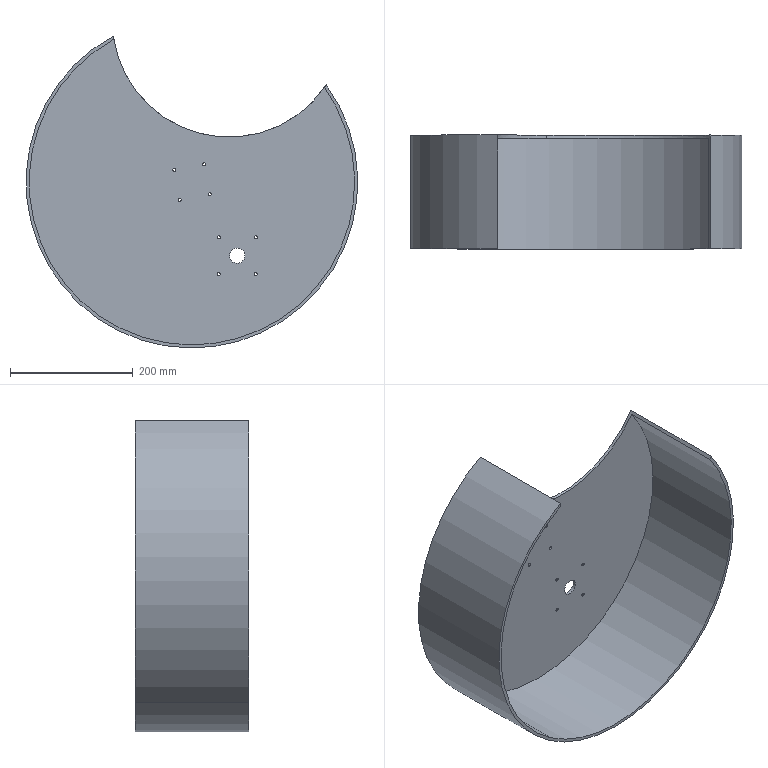Part | STEP file | Cut-Extrude 6-1 | 1 solid | 27 faces | box 540 x 185 x 507.759 mm | volume 2066014 mm3 | cylinder 24 | plane 3 | commonest cylinder face diameters 5 x16 25 x2 380 x2 530 x2 540 x2
STEP:
#1=CARTESIAN_POINT('',(-1346.779,1658.264,3090.615));
#2=VERTEX_POINT('',#1);
#3=CARTESIAN_POINT('',(-1713.217,1658.264,2718.76));
#4=VERTEX_POINT('',#3);
#5=CARTESIAN_POINT('',(-1562.535,1658.264,2936.751));
#6=DIRECTION('',(0.,1.,0.));
#7=DIRECTION('',(-0.5686,0.,-0.8226));
#8=AXIS2_PLACEMENT_3D('',#5,#6,#7);
#9=CIRCLE('',#8,265.);
#10=EDGE_CURVE('',#2,#4,#9,.T.);
#11=ORIENTED_EDGE('',*,*,#10,.T.);
#12=CARTESIAN_POINT('',(-1713.217,1478.264,2718.76));
#13=VERTEX_POINT('',#12);
#14=CARTESIAN_POINT('',(-1713.217,1658.264,2718.76));
#15=DIRECTION('',(0.,-1.,0.));
#16=VECTOR('',#15,1000.);
#17=LINE('',#14,#16);
#18=EDGE_CURVE('',#4,#13,#17,.T.);
#19=ORIENTED_EDGE('',*,*,#18,.T.);
#20=CARTESIAN_POINT('',(-1346.779,1478.264,3090.615));
#21=VERTEX_POINT('',#20);
#22=CARTESIAN_POINT('',(-1562.535,1478.264,2936.751));
#23=DIRECTION('',(0.,1.,0.));
#24=DIRECTION('',(-0.5686,0.,-0.8226));
#25=AXIS2_PLACEMENT_3D('',#22,#23,#24);
#26=CIRCLE('',#25,265.);
#27=EDGE_CURVE('',#21,#13,#26,.T.);
#28=ORIENTED_EDGE('',*,*,#27,.F.);
#29=CARTESIAN_POINT('',(-1346.779,1525.264,3090.615));
#30=DIRECTION('',(0.,-1.,0.));
#31=VECTOR('',#30,1000.);
#32=LINE('',#29,#31);
#33=EDGE_CURVE('',#2,#21,#32,.T.);
#34=ORIENTED_EDGE('',*,*,#33,.F.);
#35=EDGE_LOOP('',(#11,#19,#28,#34));
#36=FACE_OUTER_BOUND('',#35,.T.);
#37=CARTESIAN_POINT('',(-1562.535,1658.264,2936.751));
#38=DIRECTION('',(0.,-1.,0.));
#39=DIRECTION('',(-0.5686,0.,-0.8226));
#40=AXIS2_PLACEMENT_3D('',#37,#38,#39);
#41=CYLINDRICAL_SURFACE('',#40,265.);
#42=ADVANCED_FACE('',(#36),#41,.F.);
#43=CARTESIAN_POINT('',(-1716.06,1663.264,2714.647));
#44=VERTEX_POINT('',#43);
#45=CARTESIAN_POINT('',(-1690.482,1663.264,3174.51));
#46=VERTEX_POINT('',#45);
#47=CARTESIAN_POINT('',(-1562.535,1663.264,2936.751));
#48=DIRECTION('',(0.,1.,0.));
#49=DIRECTION('',(-0.5686,0.,-0.8226));
#50=AXIS2_PLACEMENT_3D('',#47,#48,#49);
#51=CIRCLE('',#50,270.);
#52=EDGE_CURVE('',#44,#46,#51,.T.);
#53=ORIENTED_EDGE('',*,*,#52,.F.);
#54=CARTESIAN_POINT('',(-1716.06,1478.264,2714.647));
#55=VERTEX_POINT('',#54);
#56=CARTESIAN_POINT('',(-1716.06,1658.264,2714.647));
#57=DIRECTION('',(0.,-1.,0.));
#58=VECTOR('',#57,1000.);
#59=LINE('',#56,#58);
#60=EDGE_CURVE('',#44,#55,#59,.T.);
#61=ORIENTED_EDGE('',*,*,#60,.T.);
#62=CARTESIAN_POINT('',(-1690.482,1478.264,3174.51));
#63=VERTEX_POINT('',#62);
#64=CARTESIAN_POINT('',(-1562.535,1478.264,2936.751));
#65=DIRECTION('',(0.,1.,0.));
#66=DIRECTION('',(-0.5686,0.,-0.8226));
#67=AXIS2_PLACEMENT_3D('',#64,#65,#66);
#68=CIRCLE('',#67,270.);
#69=EDGE_CURVE('',#55,#63,#68,.T.);
#70=ORIENTED_EDGE('',*,*,#69,.T.);
#71=CARTESIAN_POINT('',(-1690.482,1525.264,3174.51));
#72=DIRECTION('',(0.,1.,0.));
#73=VECTOR('',#72,1000.);
#74=LINE('',#71,#73);
#75=EDGE_CURVE('',#63,#46,#74,.T.);
#76=ORIENTED_EDGE('',*,*,#75,.T.);
#77=EDGE_LOOP('',(#53,#61,#70,#76));
#78=FACE_OUTER_BOUND('',#77,.T.);
#79=CARTESIAN_POINT('',(-1562.535,1658.264,2936.751));
#80=DIRECTION('',(0.,-1.,0.));
#81=DIRECTION('',(-0.5686,0.,-0.8226));
#82=AXIS2_PLACEMENT_3D('',#79,#80,#81);
#83=CYLINDRICAL_SURFACE('',#82,270.);
#84=ADVANCED_FACE('',(#78),#83,.T.);
#85=CARTESIAN_POINT('',(-1481.631,1658.264,2827.033));
#86=VERTEX_POINT('',#85);
#87=CARTESIAN_POINT('',(-1495.846,1658.264,2806.468));
#88=VERTEX_POINT('',#87);
#89=CARTESIAN_POINT('',(-1488.738,1658.264,2816.751));
#90=DIRECTION('',(0.,1.,0.));
#91=DIRECTION('',(-0.5686,0.,-0.8226));
#92=AXIS2_PLACEMENT_3D('',#89,#90,#91);
#93=CIRCLE('',#92,12.5);
#94=EDGE_CURVE('',#86,#88,#93,.T.);
#95=ORIENTED_EDGE('',*,*,#94,.F.);
#96=CARTESIAN_POINT('',(-1481.631,1663.264,2827.033));
#97=VERTEX_POINT('',#96);
#98=CARTESIAN_POINT('',(-1481.631,1653.264,2827.033));
#99=DIRECTION('',(0.,1.,0.));
#100=VECTOR('',#99,1000.);
#101=LINE('',#98,#100);
#102=EDGE_CURVE('',#86,#97,#101,.T.);
#103=ORIENTED_EDGE('',*,*,#102,.T.);
#104=CARTESIAN_POINT('',(-1495.846,1663.264,2806.468));
#105=VERTEX_POINT('',#104);
#106=CARTESIAN_POINT('',(-1488.738,1663.264,2816.751));
#107=DIRECTION('',(0.,1.,0.));
#108=DIRECTION('',(-0.5686,0.,-0.8226));
#109=AXIS2_PLACEMENT_3D('',#106,#107,#108);
#110=CIRCLE('',#109,12.5);
#111=EDGE_CURVE('',#97,#105,#110,.T.);
#112=ORIENTED_EDGE('',*,*,#111,.T.);
#113=CARTESIAN_POINT('',(-1495.846,1653.264,2806.468));
#114=DIRECTION('',(0.,1.,0.));
#115=VECTOR('',#114,1000.);
#116=LINE('',#113,#115);
#117=EDGE_CURVE('',#88,#105,#116,.T.);
#118=ORIENTED_EDGE('',*,*,#117,.F.);
#119=EDGE_LOOP('',(#95,#103,#112,#118));
#120=FACE_OUTER_BOUND('',#119,.T.);
#121=CARTESIAN_POINT('',(-1488.738,1653.264,2816.751));
#122=DIRECTION('',(0.,1.,0.));
#123=DIRECTION('',(0.5686,0.,0.8226));
#124=AXIS2_PLACEMENT_3D('',#121,#122,#123);
#125=CYLINDRICAL_SURFACE('',#124,12.5);
#126=ADVANCED_FACE('',(#120),#125,.F.);
#127=CARTESIAN_POINT('',(-1457.317,1658.264,2788.807));
#128=VERTEX_POINT('',#127);
#129=CARTESIAN_POINT('',(-1460.16,1658.264,2784.694));
#130=VERTEX_POINT('',#129);
#131=CARTESIAN_POINT('',(-1458.738,1658.264,2786.751));
#132=DIRECTION('',(0.,1.,0.));
#133=DIRECTION('',(-0.5686,0.,-0.8226));
#134=AXIS2_PLACEMENT_3D('',#131,#132,#133);
#135=CIRCLE('',#134,2.5);
#136=EDGE_CURVE('',#128,#130,#135,.T.);
#137=ORIENTED_EDGE('',*,*,#136,.F.);
#138=CARTESIAN_POINT('',(-1457.317,1663.264,2788.807));
#139=VERTEX_POINT('',#138);
#140=CARTESIAN_POINT('',(-1457.317,1663.264,2788.807));
#141=DIRECTION('',(0.,1.,0.));
#142=VECTOR('',#141,1000.);
#143=LINE('',#140,#142);
#144=EDGE_CURVE('',#128,#139,#143,.T.);
#145=ORIENTED_EDGE('',*,*,#144,.T.);
#146=CARTESIAN_POINT('',(-1460.16,1663.264,2784.694));
#147=VERTEX_POINT('',#146);
#148=CARTESIAN_POINT('',(-1458.738,1663.264,2786.751));
#149=DIRECTION('',(0.,1.,0.));
#150=DIRECTION('',(-0.5686,0.,-0.8226));
#151=AXIS2_PLACEMENT_3D('',#148,#149,#150);
#152=CIRCLE('',#151,2.5);
#153=EDGE_CURVE('',#139,#147,#152,.T.);
#154=ORIENTED_EDGE('',*,*,#153,.T.);
#155=CARTESIAN_POINT('',(-1460.16,1663.264,2784.694));
#156=DIRECTION('',(0.,1.,0.));
#157=VECTOR('',#156,1000.);
#158=LINE('',#155,#157);
#159=EDGE_CURVE('',#130,#147,#158,.T.);
#160=ORIENTED_EDGE('',*,*,#159,.F.);
#161=EDGE_LOOP('',(#137,#145,#154,#160));
#162=FACE_OUTER_BOUND('',#161,.T.);
#163=CARTESIAN_POINT('',(-1458.738,1663.264,2786.751));
#164=DIRECTION('',(0.,1.,0.));
#165=DIRECTION('',(0.5686,0.,0.8226));
#166=AXIS2_PLACEMENT_3D('',#163,#164,#165);
#167=CYLINDRICAL_SURFACE('',#166,2.5);
#168=ADVANCED_FACE('',(#162),#167,.F.);
#169=CARTESIAN_POINT('',(-1457.317,1658.264,2848.807));
#170=VERTEX_POINT('',#169);
#171=CARTESIAN_POINT('',(-1460.16,1658.264,2844.694));
#172=VERTEX_POINT('',#171);
#173=CARTESIAN_POINT('',(-1458.738,1658.264,2846.751));
#174=DIRECTION('',(0.,1.,0.));
#175=DIRECTION('',(-0.5686,0.,-0.8226));
#176=AXIS2_PLACEMENT_3D('',#173,#174,#175);
#177=CIRCLE('',#176,2.5);
#178=EDGE_CURVE('',#170,#172,#177,.T.);
#179=ORIENTED_EDGE('',*,*,#178,.F.);
#180=CARTESIAN_POINT('',(-1457.317,1663.264,2848.807));
#181=VERTEX_POINT('',#180);
#182=CARTESIAN_POINT('',(-1457.317,1663.264,2848.807));
#183=DIRECTION('',(0.,1.,0.));
#184=VECTOR('',#183,1000.);
#185=LINE('',#182,#184);
#186=EDGE_CURVE('',#170,#181,#185,.T.);
#187=ORIENTED_EDGE('',*,*,#186,.T.);
#188=CARTESIAN_POINT('',(-1460.16,1663.264,2844.694));
#189=VERTEX_POINT('',#188);
#190=CARTESIAN_POINT('',(-1458.738,1663.264,2846.751));
#191=DIRECTION('',(0.,1.,0.));
#192=DIRECTION('',(-0.5686,0.,-0.8226));
#193=AXIS2_PLACEMENT_3D('',#190,#191,#192);
#194=CIRCLE('',#193,2.5);
#195=EDGE_CURVE('',#181,#189,#194,.T.);
#196=ORIENTED_EDGE('',*,*,#195,.T.);
#197=CARTESIAN_POINT('',(-1460.16,1663.264,2844.694));
#198=DIRECTION('',(0.,1.,0.));
#199=VECTOR('',#198,1000.);
#200=LINE('',#197,#199);
#201=EDGE_CURVE('',#172,#189,#200,.T.);
#202=ORIENTED_EDGE('',*,*,#201,.F.);
#203=EDGE_LOOP('',(#179,#187,#196,#202));
#204=FACE_OUTER_BOUND('',#203,.T.);
#205=CARTESIAN_POINT('',(-1458.738,1663.264,2846.751));
#206=DIRECTION('',(0.,1.,0.));
#207=DIRECTION('',(0.5686,0.,0.8226));
#208=AXIS2_PLACEMENT_3D('',#205,#206,#207);
#209=CYLINDRICAL_SURFACE('',#208,2.5);
#210=ADVANCED_FACE('',(#204),#209,.F.);
#211=CARTESIAN_POINT('',(-1517.317,1658.264,2848.807));
#212=VERTEX_POINT('',#211);
#213=CARTESIAN_POINT('',(-1520.16,1658.264,2844.694));
#214=VERTEX_POINT('',#213);
#215=CARTESIAN_POINT('',(-1518.738,1658.264,2846.751));
#216=DIRECTION('',(0.,1.,0.));
#217=DIRECTION('',(-0.5686,0.,-0.8226));
#218=AXIS2_PLACEMENT_3D('',#215,#216,#217);
#219=CIRCLE('',#218,2.5);
#220=EDGE_CURVE('',#212,#214,#219,.T.);
#221=ORIENTED_EDGE('',*,*,#220,.F.);
#222=CARTESIAN_POINT('',(-1517.317,1663.264,2848.807));
#223=VERTEX_POINT('',#222);
#224=CARTESIAN_POINT('',(-1517.317,1663.264,2848.807));
#225=DIRECTION('',(0.,1.,0.));
#226=VECTOR('',#225,1000.);
#227=LINE('',#224,#226);
#228=EDGE_CURVE('',#212,#223,#227,.T.);
#229=ORIENTED_EDGE('',*,*,#228,.T.);
#230=CARTESIAN_POINT('',(-1520.16,1663.264,2844.694));
#231=VERTEX_POINT('',#230);
#232=CARTESIAN_POINT('',(-1518.738,1663.264,2846.751));
#233=DIRECTION('',(0.,1.,0.));
#234=DIRECTION('',(-0.5686,0.,-0.8226));
#235=AXIS2_PLACEMENT_3D('',#232,#233,#234);
#236=CIRCLE('',#235,2.5);
#237=EDGE_CURVE('',#223,#231,#236,.T.);
#238=ORIENTED_EDGE('',*,*,#237,.T.);
#239=CARTESIAN_POINT('',(-1520.16,1663.264,2844.694));
#240=DIRECTION('',(0.,1.,0.));
#241=VECTOR('',#240,1000.);
#242=LINE('',#239,#241);
#243=EDGE_CURVE('',#214,#231,#242,.T.);
#244=ORIENTED_EDGE('',*,*,#243,.F.);
#245=EDGE_LOOP('',(#221,#229,#238,#244));
#246=FACE_OUTER_BOUND('',#245,.T.);
#247=CARTESIAN_POINT('',(-1518.738,1663.264,2846.751));
#248=DIRECTION('',(0.,1.,0.));
#249=DIRECTION('',(0.5686,0.,0.8226));
#250=AXIS2_PLACEMENT_3D('',#247,#248,#249);
#251=CYLINDRICAL_SURFACE('',#250,2.5);
#252=ADVANCED_FACE('',(#246),#251,.F.);
#253=CARTESIAN_POINT('',(-1517.317,1658.264,2788.807));
#254=VERTEX_POINT('',#253);
#255=CARTESIAN_POINT('',(-1520.16,1658.264,2784.694));
#256=VERTEX_POINT('',#255);
#257=CARTESIAN_POINT('',(-1518.738,1658.264,2786.751));
#258=DIRECTION('',(0.,1.,0.));
#259=DIRECTION('',(-0.5686,0.,-0.8226));
#260=AXIS2_PLACEMENT_3D('',#257,#258,#259);
#261=CIRCLE('',#260,2.5);
#262=EDGE_CURVE('',#254,#256,#261,.T.);
#263=ORIENTED_EDGE('',*,*,#262,.F.);
#264=CARTESIAN_POINT('',(-1517.317,1663.264,2788.807));
#265=VERTEX_POINT('',#264);
#266=CARTESIAN_POINT('',(-1517.317,1663.264,2788.807));
#267=DIRECTION('',(0.,1.,0.));
#268=VECTOR('',#267,1000.);
#269=LINE('',#266,#268);
#270=EDGE_CURVE('',#254,#265,#269,.T.);
#271=ORIENTED_EDGE('',*,*,#270,.T.);
#272=CARTESIAN_POINT('',(-1520.16,1663.264,2784.694));
#273=VERTEX_POINT('',#272);
#274=CARTESIAN_POINT('',(-1518.738,1663.264,2786.751));
#275=DIRECTION('',(0.,1.,0.));
#276=DIRECTION('',(-0.5686,0.,-0.8226));
#277=AXIS2_PLACEMENT_3D('',#274,#275,#276);
#278=CIRCLE('',#277,2.5);
#279=EDGE_CURVE('',#265,#273,#278,.T.);
#280=ORIENTED_EDGE('',*,*,#279,.T.);
#281=CARTESIAN_POINT('',(-1520.16,1663.264,2784.694));
#282=DIRECTION('',(0.,1.,0.));
#283=VECTOR('',#282,1000.);
#284=LINE('',#281,#283);
#285=EDGE_CURVE('',#256,#273,#284,.T.);
#286=ORIENTED_EDGE('',*,*,#285,.F.);
#287=EDGE_LOOP('',(#263,#271,#280,#286));
#288=FACE_OUTER_BOUND('',#287,.T.);
#289=CARTESIAN_POINT('',(-1518.738,1663.264,2786.751));
#290=DIRECTION('',(0.,1.,0.));
#291=DIRECTION('',(0.5686,0.,0.8226));
#292=AXIS2_PLACEMENT_3D('',#289,#290,#291);
#293=CYLINDRICAL_SURFACE('',#292,2.5);
#294=ADVANCED_FACE('',(#288),#293,.F.);
#295=CARTESIAN_POINT('',(-1610.225,1658.264,3043.625));
#296=VERTEX_POINT('',#295);
#297=CARTESIAN_POINT('',(-1689.697,1658.264,3169.248));
#298=VERTEX_POINT('',#297);
#299=CARTESIAN_POINT('',(-1502.189,1658.264,3199.921));
#300=DIRECTION('',(0.,1.,0.));
#301=DIRECTION('',(-0.5686,0.,-0.8226));
#302=AXIS2_PLACEMENT_3D('',#299,#300,#301);
#303=CIRCLE('',#302,190.);
#304=EDGE_CURVE('',#296,#298,#303,.T.);
#305=ORIENTED_EDGE('',*,*,#304,.F.);
#306=CARTESIAN_POINT('',(-1610.225,1663.264,3043.625));
#307=VERTEX_POINT('',#306);
#308=CARTESIAN_POINT('',(-1610.225,1387.264,3043.625));
#309=DIRECTION('',(0.,1.,0.));
#310=VECTOR('',#309,1000.);
#311=LINE('',#308,#310);
#312=EDGE_CURVE('',#296,#307,#311,.T.);
#313=ORIENTED_EDGE('',*,*,#312,.T.);
#314=CARTESIAN_POINT('',(-1502.189,1663.264,3199.921));
#315=DIRECTION('',(0.,1.,0.));
#316=DIRECTION('',(-0.5686,0.,-0.8226));
#317=AXIS2_PLACEMENT_3D('',#314,#315,#316);
#318=CIRCLE('',#317,190.);
#319=EDGE_CURVE('',#307,#46,#318,.T.);
#320=ORIENTED_EDGE('',*,*,#319,.T.);
#321=ORIENTED_EDGE('',*,*,#75,.F.);
#322=CARTESIAN_POINT('',(-1689.697,1478.264,3169.248));
#323=VERTEX_POINT('',#322);
#324=CARTESIAN_POINT('',(-1502.189,1478.264,3199.921));
#325=DIRECTION('',(0.,1.,0.));
#326=DIRECTION('',(-0.5686,0.,-0.8226));
#327=AXIS2_PLACEMENT_3D('',#324,#325,#326);
#328=CIRCLE('',#327,190.);
#329=EDGE_CURVE('',#323,#63,#328,.T.);
#330=ORIENTED_EDGE('',*,*,#329,.F.);
#331=CARTESIAN_POINT('',(-1689.697,1525.264,3169.248));
#332=DIRECTION('',(0.,1.,0.));
#333=VECTOR('',#332,1000.);
#334=LINE('',#331,#333);
#335=EDGE_CURVE('',#323,#298,#334,.T.);
#336=ORIENTED_EDGE('',*,*,#335,.T.);
#337=EDGE_LOOP('',(#305,#313,#320,#321,#330,#336));
#338=FACE_OUTER_BOUND('',#337,.T.);
#339=CARTESIAN_POINT('',(-1502.189,1387.264,3199.921));
#340=DIRECTION('',(0.,1.,0.));
#341=DIRECTION('',(0.5686,0.,0.8226));
#342=AXIS2_PLACEMENT_3D('',#339,#340,#341);
#343=CYLINDRICAL_SURFACE('',#342,190.);
#344=ADVANCED_FACE('',(#338),#343,.F.);
#345=CARTESIAN_POINT('',(-1541.213,1663.264,2967.598));
#346=VERTEX_POINT('',#345);
#347=CARTESIAN_POINT('',(-1544.056,1663.264,2963.485));
#348=VERTEX_POINT('',#347);
#349=CARTESIAN_POINT('',(-1542.634,1663.264,2965.542));
#350=DIRECTION('',(0.,1.,0.));
#351=DIRECTION('',(-0.5686,0.,-0.8226));
#352=AXIS2_PLACEMENT_3D('',#349,#350,#351);
#353=CIRCLE('',#352,2.5);
#354=EDGE_CURVE('',#346,#348,#353,.T.);
#355=ORIENTED_EDGE('',*,*,#354,.T.);
#356=CARTESIAN_POINT('',(-1544.056,1658.264,2963.485));
#357=VERTEX_POINT('',#356);
#358=CARTESIAN_POINT('',(-1544.056,1658.264,2963.485));
#359=DIRECTION('',(0.,1.,0.));
#360=VECTOR('',#359,1000.);
#361=LINE('',#358,#360);
#362=EDGE_CURVE('',#357,#348,#361,.T.);
#363=ORIENTED_EDGE('',*,*,#362,.F.);
#364=CARTESIAN_POINT('',(-1541.213,1658.264,2967.598));
#365=VERTEX_POINT('',#364);
#366=CARTESIAN_POINT('',(-1542.634,1658.264,2965.542));
#367=DIRECTION('',(0.,-1.,0.));
#368=DIRECTION('',(0.5686,0.,0.8226));
#369=AXIS2_PLACEMENT_3D('',#366,#367,#368);
#370=CIRCLE('',#369,2.5);
#371=EDGE_CURVE('',#357,#365,#370,.T.);
#372=ORIENTED_EDGE('',*,*,#371,.T.);
#373=CARTESIAN_POINT('',(-1541.213,1658.264,2967.598));
#374=DIRECTION('',(0.,1.,0.));
#375=VECTOR('',#374,1000.);
#376=LINE('',#373,#375);
#377=EDGE_CURVE('',#365,#346,#376,.T.);
#378=ORIENTED_EDGE('',*,*,#377,.T.);
#379=EDGE_LOOP('',(#355,#363,#372,#378));
#380=FACE_OUTER_BOUND('',#379,.T.);
#381=CARTESIAN_POINT('',(-1542.634,1658.264,2965.542));
#382=DIRECTION('',(0.,-1.,0.));
#383=DIRECTION('',(-0.5686,0.,-0.8226));
#384=AXIS2_PLACEMENT_3D('',#381,#382,#383);
#385=CYLINDRICAL_SURFACE('',#384,2.5);
#386=ADVANCED_FACE('',(#380),#385,.F.);
#387=CARTESIAN_POINT('',(-1589.905,1663.264,2958.709));
#388=VERTEX_POINT('',#387);
#389=CARTESIAN_POINT('',(-1592.748,1663.264,2954.596));
#390=VERTEX_POINT('',#389);
#391=CARTESIAN_POINT('',(-1591.327,1663.264,2956.652));
#392=DIRECTION('',(0.,1.,0.));
#393=DIRECTION('',(-0.5686,0.,-0.8226));
#394=AXIS2_PLACEMENT_3D('',#391,#392,#393);
#395=CIRCLE('',#394,2.5);
#396=EDGE_CURVE('',#388,#390,#395,.T.);
#397=ORIENTED_EDGE('',*,*,#396,.T.);
#398=CARTESIAN_POINT('',(-1592.748,1658.264,2954.596));
#399=VERTEX_POINT('',#398);
#400=CARTESIAN_POINT('',(-1592.748,1658.264,2954.596));
#401=DIRECTION('',(0.,1.,0.));
#402=VECTOR('',#401,1000.);
#403=LINE('',#400,#402);
#404=EDGE_CURVE('',#399,#390,#403,.T.);
#405=ORIENTED_EDGE('',*,*,#404,.F.);
#406=CARTESIAN_POINT('',(-1589.905,1658.264,2958.709));
#407=VERTEX_POINT('',#406);
#408=CARTESIAN_POINT('',(-1591.327,1658.264,2956.652));
#409=DIRECTION('',(0.,-1.,0.));
#410=DIRECTION('',(0.5686,0.,0.8226));
#411=AXIS2_PLACEMENT_3D('',#408,#409,#410);
#412=CIRCLE('',#411,2.5);
#413=EDGE_CURVE('',#399,#407,#412,.T.);
#414=ORIENTED_EDGE('',*,*,#413,.T.);
#415=CARTESIAN_POINT('',(-1589.905,1658.264,2958.709));
#416=DIRECTION('',(0.,1.,0.));
#417=VECTOR('',#416,1000.);
#418=LINE('',#415,#417);
#419=EDGE_CURVE('',#407,#388,#418,.T.);
#420=ORIENTED_EDGE('',*,*,#419,.T.);
#421=EDGE_LOOP('',(#397,#405,#414,#420));
#422=FACE_OUTER_BOUND('',#421,.T.);
#423=CARTESIAN_POINT('',(-1591.327,1658.264,2956.652));
#424=DIRECTION('',(0.,-1.,0.));
#425=DIRECTION('',(-0.5686,0.,-0.8226));
#426=AXIS2_PLACEMENT_3D('',#423,#424,#425);
#427=CYLINDRICAL_SURFACE('',#426,2.5);
#428=ADVANCED_FACE('',(#422),#427,.F.);
#429=CARTESIAN_POINT('',(-1532.323,1663.264,2918.906));
#430=VERTEX_POINT('',#429);
#431=CARTESIAN_POINT('',(-1535.166,1663.264,2914.793));
#432=VERTEX_POINT('',#431);
#433=CARTESIAN_POINT('',(-1533.744,1663.264,2916.849));
#434=DIRECTION('',(0.,1.,0.));
#435=DIRECTION('',(-0.5686,0.,-0.8226));
#436=AXIS2_PLACEMENT_3D('',#433,#434,#435);
#437=CIRCLE('',#436,2.5);
#438=EDGE_CURVE('',#430,#432,#437,.T.);
#439=ORIENTED_EDGE('',*,*,#438,.T.);
#440=CARTESIAN_POINT('',(-1535.166,1658.264,2914.793));
#441=VERTEX_POINT('',#440);
#442=CARTESIAN_POINT('',(-1535.166,1658.264,2914.793));
#443=DIRECTION('',(0.,1.,0.));
#444=VECTOR('',#443,1000.);
#445=LINE('',#442,#444);
#446=EDGE_CURVE('',#441,#432,#445,.T.);
#447=ORIENTED_EDGE('',*,*,#446,.F.);
#448=CARTESIAN_POINT('',(-1532.323,1658.264,2918.906));
#449=VERTEX_POINT('',#448);
#450=CARTESIAN_POINT('',(-1533.744,1658.264,2916.849));
#451=DIRECTION('',(0.,-1.,0.));
#452=DIRECTION('',(0.5686,0.,0.8226));
#453=AXIS2_PLACEMENT_3D('',#450,#451,#452);
#454=CIRCLE('',#453,2.5);
#455=EDGE_CURVE('',#441,#449,#454,.T.);
#456=ORIENTED_EDGE('',*,*,#455,.T.);
#457=CARTESIAN_POINT('',(-1532.323,1658.264,2918.906));
#458=DIRECTION('',(0.,1.,0.));
#459=VECTOR('',#458,1000.);
#460=LINE('',#457,#459);
#461=EDGE_CURVE('',#449,#430,#460,.T.);
#462=ORIENTED_EDGE('',*,*,#461,.T.);
#463=EDGE_LOOP('',(#439,#447,#456,#462));
#464=FACE_OUTER_BOUND('',#463,.T.);
#465=CARTESIAN_POINT('',(-1533.744,1658.264,2916.849));
#466=DIRECTION('',(0.,-1.,0.));
#467=DIRECTION('',(-0.5686,0.,-0.8226));
#468=AXIS2_PLACEMENT_3D('',#465,#466,#467);
#469=CYLINDRICAL_SURFACE('',#468,2.5);
#470=ADVANCED_FACE('',(#464),#469,.F.);
#471=CARTESIAN_POINT('',(-1581.015,1663.264,2910.016));
#472=VERTEX_POINT('',#471);
#473=CARTESIAN_POINT('',(-1583.858,1663.264,2905.903));
#474=VERTEX_POINT('',#473);
#475=CARTESIAN_POINT('',(-1582.437,1663.264,2907.959));
#476=DIRECTION('',(0.,1.,0.));
#477=DIRECTION('',(-0.5686,0.,-0.8226));
#478=AXIS2_PLACEMENT_3D('',#475,#476,#477);
#479=CIRCLE('',#478,2.5);
#480=EDGE_CURVE('',#472,#474,#479,.T.);
#481=ORIENTED_EDGE('',*,*,#480,.T.);
#482=CARTESIAN_POINT('',(-1583.858,1658.264,2905.903));
#483=VERTEX_POINT('',#482);
#484=CARTESIAN_POINT('',(-1583.858,1658.264,2905.903));
#485=DIRECTION('',(0.,1.,0.));
#486=VECTOR('',#485,1000.);
#487=LINE('',#484,#486);
#488=EDGE_CURVE('',#483,#474,#487,.T.);
#489=ORIENTED_EDGE('',*,*,#488,.F.);
#490=CARTESIAN_POINT('',(-1581.015,1658.264,2910.016));
#491=VERTEX_POINT('',#490);
#492=CARTESIAN_POINT('',(-1582.437,1658.264,2907.959));
#493=DIRECTION('',(0.,-1.,0.));
#494=DIRECTION('',(0.5686,0.,0.8226));
#495=AXIS2_PLACEMENT_3D('',#492,#493,#494);
#496=CIRCLE('',#495,2.5);
#497=EDGE_CURVE('',#483,#491,#496,.T.);
#498=ORIENTED_EDGE('',*,*,#497,.T.);
#499=CARTESIAN_POINT('',(-1581.015,1658.264,2910.016));
#500=DIRECTION('',(0.,1.,0.));
#501=VECTOR('',#500,1000.);
#502=LINE('',#499,#501);
#503=EDGE_CURVE('',#491,#472,#502,.T.);
#504=ORIENTED_EDGE('',*,*,#503,.T.);
#505=EDGE_LOOP('',(#481,#489,#498,#504));
#506=FACE_OUTER_BOUND('',#505,.T.);
#507=CARTESIAN_POINT('',(-1582.437,1658.264,2907.959));
#508=DIRECTION('',(0.,-1.,0.));
#509=DIRECTION('',(-0.5686,0.,-0.8226));
#510=AXIS2_PLACEMENT_3D('',#507,#508,#509);
#511=CYLINDRICAL_SURFACE('',#510,2.5);
#512=ADVANCED_FACE('',(#506),#511,.F.);
#513=ORIENTED_EDGE('',*,*,#60,.F.);
#514=CARTESIAN_POINT('',(-1343.779,1663.264,3095.009));
#515=VERTEX_POINT('',#514);
#516=CARTESIAN_POINT('',(-1562.535,1663.264,2936.751));
#517=DIRECTION('',(0.,1.,0.));
#518=DIRECTION('',(-0.5686,0.,-0.8226));
#519=AXIS2_PLACEMENT_3D('',#516,#517,#518);
#520=CIRCLE('',#519,270.);
#521=EDGE_CURVE('',#515,#44,#520,.T.);
#522=ORIENTED_EDGE('',*,*,#521,.F.);
#523=CARTESIAN_POINT('',(-1343.779,1478.264,3095.009));
#524=VERTEX_POINT('',#523);
#525=CARTESIAN_POINT('',(-1343.779,1525.264,3095.009));
#526=DIRECTION('',(0.,-1.,0.));
#527=VECTOR('',#526,1000.);
#528=LINE('',#525,#527);
#529=EDGE_CURVE('',#515,#524,#528,.T.);
#530=ORIENTED_EDGE('',*,*,#529,.T.);
#531=CARTESIAN_POINT('',(-1562.535,1478.264,2936.751));
#532=DIRECTION('',(0.,1.,0.));
#533=DIRECTION('',(-0.5686,0.,-0.8226));
#534=AXIS2_PLACEMENT_3D('',#531,#532,#533);
#535=CIRCLE('',#534,270.);
#536=EDGE_CURVE('',#524,#55,#535,.T.);
#537=ORIENTED_EDGE('',*,*,#536,.T.);
#538=EDGE_LOOP('',(#513,#522,#530,#537));
#539=FACE_OUTER_BOUND('',#538,.T.);
#540=CARTESIAN_POINT('',(-1562.535,1658.264,2936.751));
#541=DIRECTION('',(0.,-1.,0.));
#542=DIRECTION('',(-0.5686,0.,-0.8226));
#543=AXIS2_PLACEMENT_3D('',#540,#541,#542);
#544=CYLINDRICAL_SURFACE('',#543,270.);
#545=ADVANCED_FACE('',(#539),#544,.T.);
#546=CARTESIAN_POINT('',(-1488.738,1663.264,2816.751));
#547=DIRECTION('',(0.,1.,0.));
#548=DIRECTION('',(-0.5686,0.,-0.8226));
#549=AXIS2_PLACEMENT_3D('',#546,#547,#548);
#550=CIRCLE('',#549,12.5);
#551=EDGE_CURVE('',#105,#97,#550,.T.);
#552=ORIENTED_EDGE('',*,*,#551,.F.);
#553=ORIENTED_EDGE('',*,*,#111,.F.);
#554=EDGE_LOOP('',(#552,#553));
#555=FACE_BOUND('',#554,.T.);
#556=CARTESIAN_POINT('',(-1458.738,1663.264,2786.751));
#557=DIRECTION('',(0.,1.,0.));
#558=DIRECTION('',(-0.5686,0.,-0.8226));
#559=AXIS2_PLACEMENT_3D('',#556,#557,#558);
#560=CIRCLE('',#559,2.5);
#561=EDGE_CURVE('',#147,#139,#560,.T.);
#562=ORIENTED_EDGE('',*,*,#561,.F.);
#563=ORIENTED_EDGE('',*,*,#153,.F.);
#564=EDGE_LOOP('',(#562,#563));
#565=FACE_BOUND('',#564,.T.);
#566=CARTESIAN_POINT('',(-1458.738,1663.264,2846.751));
#567=DIRECTION('',(0.,1.,0.));
#568=DIRECTION('',(-0.5686,0.,-0.8226));
#569=AXIS2_PLACEMENT_3D('',#566,#567,#568);
#570=CIRCLE('',#569,2.5);
#571=EDGE_CURVE('',#189,#181,#570,.T.);
#572=ORIENTED_EDGE('',*,*,#571,.F.);
#573=ORIENTED_EDGE('',*,*,#195,.F.);
#574=EDGE_LOOP('',(#572,#573));
#575=FACE_BOUND('',#574,.T.);
#576=CARTESIAN_POINT('',(-1518.738,1663.264,2846.751));
#577=DIRECTION('',(0.,1.,0.));
#578=DIRECTION('',(-0.5686,0.,-0.8226));
#579=AXIS2_PLACEMENT_3D('',#576,#577,#578);
#580=CIRCLE('',#579,2.5);
#581=EDGE_CURVE('',#231,#223,#580,.T.);
#582=ORIENTED_EDGE('',*,*,#581,.F.);
#583=ORIENTED_EDGE('',*,*,#237,.F.);
#584=EDGE_LOOP('',(#582,#583));
#585=FACE_BOUND('',#584,.T.);
#586=CARTESIAN_POINT('',(-1518.738,1663.264,2786.751));
#587=DIRECTION('',(0.,1.,0.));
#588=DIRECTION('',(-0.5686,0.,-0.8226));
#589=AXIS2_PLACEMENT_3D('',#586,#587,#588);
#590=CIRCLE('',#589,2.5);
#591=EDGE_CURVE('',#273,#265,#590,.T.);
#592=ORIENTED_EDGE('',*,*,#591,.F.);
#593=ORIENTED_EDGE('',*,*,#279,.F.);
#594=EDGE_LOOP('',(#592,#593));
#595=FACE_BOUND('',#594,.T.);
#596=CARTESIAN_POINT('',(-1502.189,1663.264,3199.921));
#597=DIRECTION('',(0.,1.,0.));
#598=DIRECTION('',(-0.5686,0.,-0.8226));
#599=AXIS2_PLACEMENT_3D('',#596,#597,#598);
#600=CIRCLE('',#599,190.);
#601=EDGE_CURVE('',#515,#307,#600,.T.);
#602=ORIENTED_EDGE('',*,*,#601,.F.);
#603=ORIENTED_EDGE('',*,*,#521,.T.);
#604=ORIENTED_EDGE('',*,*,#52,.T.);
#605=ORIENTED_EDGE('',*,*,#319,.F.);
#606=EDGE_LOOP('',(#602,#603,#604,#605));
#607=FACE_OUTER_BOUND('',#606,.T.);
#608=ORIENTED_EDGE('',*,*,#354,.F.);
#609=CARTESIAN_POINT('',(-1542.634,1663.264,2965.542));
#610=DIRECTION('',(0.,1.,0.));
#611=DIRECTION('',(-0.5686,0.,-0.8226));
#612=AXIS2_PLACEMENT_3D('',#609,#610,#611);
#613=CIRCLE('',#612,2.5);
#614=EDGE_CURVE('',#348,#346,#613,.T.);
#615=ORIENTED_EDGE('',*,*,#614,.F.);
#616=EDGE_LOOP('',(#608,#615));
#617=FACE_BOUND('',#616,.T.);
#618=ORIENTED_EDGE('',*,*,#396,.F.);
#619=CARTESIAN_POINT('',(-1591.327,1663.264,2956.652));
#620=DIRECTION('',(0.,1.,0.));
#621=DIRECTION('',(-0.5686,0.,-0.8226));
#622=AXIS2_PLACEMENT_3D('',#619,#620,#621);
#623=CIRCLE('',#622,2.5);
#624=EDGE_CURVE('',#390,#388,#623,.T.);
#625=ORIENTED_EDGE('',*,*,#624,.F.);
#626=EDGE_LOOP('',(#618,#625));
#627=FACE_BOUND('',#626,.T.);
#628=ORIENTED_EDGE('',*,*,#438,.F.);
#629=CARTESIAN_POINT('',(-1533.744,1663.264,2916.849));
#630=DIRECTION('',(0.,1.,0.));
#631=DIRECTION('',(-0.5686,0.,-0.8226));
#632=AXIS2_PLACEMENT_3D('',#629,#630,#631);
#633=CIRCLE('',#632,2.5);
#634=EDGE_CURVE('',#432,#430,#633,.T.);
#635=ORIENTED_EDGE('',*,*,#634,.F.);
#636=EDGE_LOOP('',(#628,#635));
#637=FACE_BOUND('',#636,.T.);
#638=ORIENTED_EDGE('',*,*,#480,.F.);
#639=CARTESIAN_POINT('',(-1582.437,1663.264,2907.959));
#640=DIRECTION('',(0.,1.,0.));
#641=DIRECTION('',(-0.5686,0.,-0.8226));
#642=AXIS2_PLACEMENT_3D('',#639,#640,#641);
#643=CIRCLE('',#642,2.5);
#644=EDGE_CURVE('',#474,#472,#643,.T.);
#645=ORIENTED_EDGE('',*,*,#644,.F.);
#646=EDGE_LOOP('',(#638,#645));
#647=FACE_BOUND('',#646,.T.);
#648=CARTESIAN_POINT('',(-1562.535,1663.264,2936.751));
#649=DIRECTION('',(0.,1.,0.));
#650=DIRECTION('',(0.5686,0.,0.8226));
#651=AXIS2_PLACEMENT_3D('',#648,#649,#650);
#652=PLANE('',#651);
#653=ADVANCED_FACE('',(#555,#565,#575,#585,#595,#607,#617,#627,#637,#647),#652,.T.);
#654=ORIENTED_EDGE('',*,*,#27,.T.);
#655=CARTESIAN_POINT('',(-1562.535,1478.264,2936.751));
#656=DIRECTION('',(0.,1.,0.));
#657=DIRECTION('',(-0.5686,0.,-0.8226));
#658=AXIS2_PLACEMENT_3D('',#655,#656,#657);
#659=CIRCLE('',#658,265.);
#660=EDGE_CURVE('',#13,#323,#659,.T.);
#661=ORIENTED_EDGE('',*,*,#660,.T.);
#662=ORIENTED_EDGE('',*,*,#329,.T.);
#663=ORIENTED_EDGE('',*,*,#69,.F.);
#664=ORIENTED_EDGE('',*,*,#536,.F.);
#665=CARTESIAN_POINT('',(-1502.189,1478.264,3199.921));
#666=DIRECTION('',(0.,1.,0.));
#667=DIRECTION('',(-0.5686,0.,-0.8226));
#668=AXIS2_PLACEMENT_3D('',#665,#666,#667);
#669=CIRCLE('',#668,190.);
#670=EDGE_CURVE('',#524,#21,#669,.T.);
#671=ORIENTED_EDGE('',*,*,#670,.T.);
#672=EDGE_LOOP('',(#654,#661,#662,#663,#664,#671));
#673=FACE_OUTER_BOUND('',#672,.T.);
#674=CARTESIAN_POINT('',(-1562.535,1478.264,2936.751));
#675=DIRECTION('',(0.,1.,0.));
#676=DIRECTION('',(0.5686,0.,0.8226));
#677=AXIS2_PLACEMENT_3D('',#674,#675,#676);
#678=PLANE('',#677);
#679=ADVANCED_FACE('',(#673),#678,.F.);
#680=ORIENTED_EDGE('',*,*,#18,.F.);
#681=CARTESIAN_POINT('',(-1562.535,1658.264,2936.751));
#682=DIRECTION('',(0.,1.,0.));
#683=DIRECTION('',(-0.5686,0.,-0.8226));
#684=AXIS2_PLACEMENT_3D('',#681,#682,#683);
#685=CIRCLE('',#684,265.);
#686=EDGE_CURVE('',#4,#298,#685,.T.);
#687=ORIENTED_EDGE('',*,*,#686,.T.);
#688=ORIENTED_EDGE('',*,*,#335,.F.);
#689=ORIENTED_EDGE('',*,*,#660,.F.);
#690=EDGE_LOOP('',(#680,#687,#688,#689));
#691=FACE_OUTER_BOUND('',#690,.T.);
#692=CARTESIAN_POINT('',(-1562.535,1658.264,2936.751));
#693=DIRECTION('',(0.,-1.,0.));
#694=DIRECTION('',(-0.5686,0.,-0.8226));
#695=AXIS2_PLACEMENT_3D('',#692,#693,#694);
#696=CYLINDRICAL_SURFACE('',#695,265.);
#697=ADVANCED_FACE('',(#691),#696,.F.);
#698=CARTESIAN_POINT('',(-1488.738,1658.264,2816.751));
#699=DIRECTION('',(0.,1.,0.));
#700=DIRECTION('',(-0.5686,0.,-0.8226));
#701=AXIS2_PLACEMENT_3D('',#698,#699,#700);
#702=CIRCLE('',#701,12.5);
#703=EDGE_CURVE('',#88,#86,#702,.T.);
#704=ORIENTED_EDGE('',*,*,#703,.T.);
#705=ORIENTED_EDGE('',*,*,#94,.T.);
#706=EDGE_LOOP('',(#704,#705));
#707=FACE_BOUND('',#706,.T.);
#708=CARTESIAN_POINT('',(-1458.738,1658.264,2786.751));
#709=DIRECTION('',(0.,1.,0.));
#710=DIRECTION('',(-0.5686,0.,-0.8226));
#711=AXIS2_PLACEMENT_3D('',#708,#709,#710);
#712=CIRCLE('',#711,2.5);
#713=EDGE_CURVE('',#130,#128,#712,.T.);
#714=ORIENTED_EDGE('',*,*,#713,.T.);
#715=ORIENTED_EDGE('',*,*,#136,.T.);
#716=EDGE_LOOP('',(#714,#715));
#717=FACE_BOUND('',#716,.T.);
#718=CARTESIAN_POINT('',(-1458.738,1658.264,2846.751));
#719=DIRECTION('',(0.,1.,0.));
#720=DIRECTION('',(-0.5686,0.,-0.8226));
#721=AXIS2_PLACEMENT_3D('',#718,#719,#720);
#722=CIRCLE('',#721,2.5);
#723=EDGE_CURVE('',#172,#170,#722,.T.);
#724=ORIENTED_EDGE('',*,*,#723,.T.);
#725=ORIENTED_EDGE('',*,*,#178,.T.);
#726=EDGE_LOOP('',(#724,#725));
#727=FACE_BOUND('',#726,.T.);
#728=CARTESIAN_POINT('',(-1518.738,1658.264,2846.751));
#729=DIRECTION('',(0.,1.,0.));
#730=DIRECTION('',(-0.5686,0.,-0.8226));
#731=AXIS2_PLACEMENT_3D('',#728,#729,#730);
#732=CIRCLE('',#731,2.5);
#733=EDGE_CURVE('',#214,#212,#732,.T.);
#734=ORIENTED_EDGE('',*,*,#733,.T.);
#735=ORIENTED_EDGE('',*,*,#220,.T.);
#736=EDGE_LOOP('',(#734,#735));
#737=FACE_BOUND('',#736,.T.);
#738=CARTESIAN_POINT('',(-1518.738,1658.264,2786.751));
#739=DIRECTION('',(0.,1.,0.));
#740=DIRECTION('',(-0.5686,0.,-0.8226));
#741=AXIS2_PLACEMENT_3D('',#738,#739,#740);
#742=CIRCLE('',#741,2.5);
#743=EDGE_CURVE('',#256,#254,#742,.T.);
#744=ORIENTED_EDGE('',*,*,#743,.T.);
#745=ORIENTED_EDGE('',*,*,#262,.T.);
#746=EDGE_LOOP('',(#744,#745));
#747=FACE_BOUND('',#746,.T.);
#748=CARTESIAN_POINT('',(-1542.634,1658.264,2965.542));
#749=DIRECTION('',(0.,-1.,0.));
#750=DIRECTION('',(0.5686,0.,0.8226));
#751=AXIS2_PLACEMENT_3D('',#748,#749,#750);
#752=CIRCLE('',#751,2.5);
#753=EDGE_CURVE('',#365,#357,#752,.T.);
#754=ORIENTED_EDGE('',*,*,#753,.F.);
#755=ORIENTED_EDGE('',*,*,#371,.F.);
#756=EDGE_LOOP('',(#754,#755));
#757=FACE_BOUND('',#756,.T.);
#758=CARTESIAN_POINT('',(-1591.327,1658.264,2956.652));
#759=DIRECTION('',(0.,-1.,0.));
#760=DIRECTION('',(0.5686,0.,0.8226));
#761=AXIS2_PLACEMENT_3D('',#758,#759,#760);
#762=CIRCLE('',#761,2.5);
#763=EDGE_CURVE('',#407,#399,#762,.T.);
#764=ORIENTED_EDGE('',*,*,#763,.F.);
#765=ORIENTED_EDGE('',*,*,#413,.F.);
#766=EDGE_LOOP('',(#764,#765));
#767=FACE_BOUND('',#766,.T.);
#768=CARTESIAN_POINT('',(-1533.744,1658.264,2916.849));
#769=DIRECTION('',(0.,-1.,0.));
#770=DIRECTION('',(0.5686,0.,0.8226));
#771=AXIS2_PLACEMENT_3D('',#768,#769,#770);
#772=CIRCLE('',#771,2.5);
#773=EDGE_CURVE('',#449,#441,#772,.T.);
#774=ORIENTED_EDGE('',*,*,#773,.F.);
#775=ORIENTED_EDGE('',*,*,#455,.F.);
#776=EDGE_LOOP('',(#774,#775));
#777=FACE_BOUND('',#776,.T.);
#778=CARTESIAN_POINT('',(-1582.437,1658.264,2907.959));
#779=DIRECTION('',(0.,-1.,0.));
#780=DIRECTION('',(0.5686,0.,0.8226));
#781=AXIS2_PLACEMENT_3D('',#778,#779,#780);
#782=CIRCLE('',#781,2.5);
#783=EDGE_CURVE('',#491,#483,#782,.T.);
#784=ORIENTED_EDGE('',*,*,#783,.F.);
#785=ORIENTED_EDGE('',*,*,#497,.F.);
#786=EDGE_LOOP('',(#784,#785));
#787=FACE_BOUND('',#786,.T.);
#788=ORIENTED_EDGE('',*,*,#10,.F.);
#789=CARTESIAN_POINT('',(-1502.189,1658.264,3199.921));
#790=DIRECTION('',(0.,1.,0.));
#791=DIRECTION('',(-0.5686,0.,-0.8226));
#792=AXIS2_PLACEMENT_3D('',#789,#790,#791);
#793=CIRCLE('',#792,190.);
#794=EDGE_CURVE('',#2,#296,#793,.T.);
#795=ORIENTED_EDGE('',*,*,#794,.T.);
#796=ORIENTED_EDGE('',*,*,#304,.T.);
#797=ORIENTED_EDGE('',*,*,#686,.F.);
#798=EDGE_LOOP('',(#788,#795,#796,#797));
#799=FACE_OUTER_BOUND('',#798,.T.);
#800=CARTESIAN_POINT('',(-1562.535,1658.264,2936.751));
#801=DIRECTION('',(0.,1.,0.));
#802=DIRECTION('',(0.5686,0.,0.8226));
#803=AXIS2_PLACEMENT_3D('',#800,#801,#802);
#804=PLANE('',#803);
#805=ADVANCED_FACE('',(#707,#717,#727,#737,#747,#757,#767,#777,#787,#799),#804,.F.);
#806=ORIENTED_EDGE('',*,*,#488,.T.);
#807=ORIENTED_EDGE('',*,*,#644,.T.);
#808=ORIENTED_EDGE('',*,*,#503,.F.);
#809=ORIENTED_EDGE('',*,*,#783,.T.);
#810=EDGE_LOOP('',(#806,#807,#808,#809));
#811=FACE_OUTER_BOUND('',#810,.T.);
#812=CARTESIAN_POINT('',(-1582.437,1658.264,2907.959));
#813=DIRECTION('',(0.,-1.,0.));
#814=DIRECTION('',(-0.5686,0.,-0.8226));
#815=AXIS2_PLACEMENT_3D('',#812,#813,#814);
#816=CYLINDRICAL_SURFACE('',#815,2.5);
#817=ADVANCED_FACE('',(#811),#816,.F.);
#818=ORIENTED_EDGE('',*,*,#446,.T.);
#819=ORIENTED_EDGE('',*,*,#634,.T.);
#820=ORIENTED_EDGE('',*,*,#461,.F.);
#821=ORIENTED_EDGE('',*,*,#773,.T.);
#822=EDGE_LOOP('',(#818,#819,#820,#821));
#823=FACE_OUTER_BOUND('',#822,.T.);
#824=CARTESIAN_POINT('',(-1533.744,1658.264,2916.849));
#825=DIRECTION('',(0.,-1.,0.));
#826=DIRECTION('',(-0.5686,0.,-0.8226));
#827=AXIS2_PLACEMENT_3D('',#824,#825,#826);
#828=CYLINDRICAL_SURFACE('',#827,2.5);
#829=ADVANCED_FACE('',(#823),#828,.F.);
#830=ORIENTED_EDGE('',*,*,#404,.T.);
#831=ORIENTED_EDGE('',*,*,#624,.T.);
#832=ORIENTED_EDGE('',*,*,#419,.F.);
#833=ORIENTED_EDGE('',*,*,#763,.T.);
#834=EDGE_LOOP('',(#830,#831,#832,#833));
#835=FACE_OUTER_BOUND('',#834,.T.);
#836=CARTESIAN_POINT('',(-1591.327,1658.264,2956.652));
#837=DIRECTION('',(0.,-1.,0.));
#838=DIRECTION('',(-0.5686,0.,-0.8226));
#839=AXIS2_PLACEMENT_3D('',#836,#837,#838);
#840=CYLINDRICAL_SURFACE('',#839,2.5);
#841=ADVANCED_FACE('',(#835),#840,.F.);
#842=ORIENTED_EDGE('',*,*,#362,.T.);
#843=ORIENTED_EDGE('',*,*,#614,.T.);
#844=ORIENTED_EDGE('',*,*,#377,.F.);
#845=ORIENTED_EDGE('',*,*,#753,.T.);
#846=EDGE_LOOP('',(#842,#843,#844,#845));
#847=FACE_OUTER_BOUND('',#846,.T.);
#848=CARTESIAN_POINT('',(-1542.634,1658.264,2965.542));
#849=DIRECTION('',(0.,-1.,0.));
#850=DIRECTION('',(-0.5686,0.,-0.8226));
#851=AXIS2_PLACEMENT_3D('',#848,#849,#850);
#852=CYLINDRICAL_SURFACE('',#851,2.5);
#853=ADVANCED_FACE('',(#847),#852,.F.);
#854=ORIENTED_EDGE('',*,*,#312,.F.);
#855=ORIENTED_EDGE('',*,*,#794,.F.);
#856=ORIENTED_EDGE('',*,*,#33,.T.);
#857=ORIENTED_EDGE('',*,*,#670,.F.);
#858=ORIENTED_EDGE('',*,*,#529,.F.);
#859=ORIENTED_EDGE('',*,*,#601,.T.);
#860=EDGE_LOOP('',(#854,#855,#856,#857,#858,#859));
#861=FACE_OUTER_BOUND('',#860,.T.);
#862=CARTESIAN_POINT('',(-1502.189,1387.264,3199.921));
#863=DIRECTION('',(0.,1.,0.));
#864=DIRECTION('',(0.5686,0.,0.8226));
#865=AXIS2_PLACEMENT_3D('',#862,#863,#864);
#866=CYLINDRICAL_SURFACE('',#865,190.);
#867=ADVANCED_FACE('',(#861),#866,.F.);
#868=ORIENTED_EDGE('',*,*,#270,.F.);
#869=ORIENTED_EDGE('',*,*,#743,.F.);
#870=ORIENTED_EDGE('',*,*,#285,.T.);
#871=ORIENTED_EDGE('',*,*,#591,.T.);
#872=EDGE_LOOP('',(#868,#869,#870,#871));
#873=FACE_OUTER_BOUND('',#872,.T.);
#874=CARTESIAN_POINT('',(-1518.738,1663.264,2786.751));
#875=DIRECTION('',(0.,1.,0.));
#876=DIRECTION('',(0.5686,0.,0.8226));
#877=AXIS2_PLACEMENT_3D('',#874,#875,#876);
#878=CYLINDRICAL_SURFACE('',#877,2.5);
#879=ADVANCED_FACE('',(#873),#878,.F.);
#880=ORIENTED_EDGE('',*,*,#228,.F.);
#881=ORIENTED_EDGE('',*,*,#733,.F.);
#882=ORIENTED_EDGE('',*,*,#243,.T.);
#883=ORIENTED_EDGE('',*,*,#581,.T.);
#884=EDGE_LOOP('',(#880,#881,#882,#883));
#885=FACE_OUTER_BOUND('',#884,.T.);
#886=CARTESIAN_POINT('',(-1518.738,1663.264,2846.751));
#887=DIRECTION('',(0.,1.,0.));
#888=DIRECTION('',(0.5686,0.,0.8226));
#889=AXIS2_PLACEMENT_3D('',#886,#887,#888);
#890=CYLINDRICAL_SURFACE('',#889,2.5);
#891=ADVANCED_FACE('',(#885),#890,.F.);
#892=ORIENTED_EDGE('',*,*,#186,.F.);
#893=ORIENTED_EDGE('',*,*,#723,.F.);
#894=ORIENTED_EDGE('',*,*,#201,.T.);
#895=ORIENTED_EDGE('',*,*,#571,.T.);
#896=EDGE_LOOP('',(#892,#893,#894,#895));
#897=FACE_OUTER_BOUND('',#896,.T.);
#898=CARTESIAN_POINT('',(-1458.738,1663.264,2846.751));
#899=DIRECTION('',(0.,1.,0.));
#900=DIRECTION('',(0.5686,0.,0.8226));
#901=AXIS2_PLACEMENT_3D('',#898,#899,#900);
#902=CYLINDRICAL_SURFACE('',#901,2.5);
#903=ADVANCED_FACE('',(#897),#902,.F.);
#904=ORIENTED_EDGE('',*,*,#144,.F.);
#905=ORIENTED_EDGE('',*,*,#713,.F.);
#906=ORIENTED_EDGE('',*,*,#159,.T.);
#907=ORIENTED_EDGE('',*,*,#561,.T.);
#908=EDGE_LOOP('',(#904,#905,#906,#907));
#909=FACE_OUTER_BOUND('',#908,.T.);
#910=CARTESIAN_POINT('',(-1458.738,1663.264,2786.751));
#911=DIRECTION('',(0.,1.,0.));
#912=DIRECTION('',(0.5686,0.,0.8226));
#913=AXIS2_PLACEMENT_3D('',#910,#911,#912);
#914=CYLINDRICAL_SURFACE('',#913,2.5);
#915=ADVANCED_FACE('',(#909),#914,.F.);
#916=ORIENTED_EDGE('',*,*,#102,.F.);
#917=ORIENTED_EDGE('',*,*,#703,.F.);
#918=ORIENTED_EDGE('',*,*,#117,.T.);
#919=ORIENTED_EDGE('',*,*,#551,.T.);
#920=EDGE_LOOP('',(#916,#917,#918,#919));
#921=FACE_OUTER_BOUND('',#920,.T.);
#922=CARTESIAN_POINT('',(-1488.738,1653.264,2816.751));
#923=DIRECTION('',(0.,1.,0.));
#924=DIRECTION('',(0.5686,0.,0.8226));
#925=AXIS2_PLACEMENT_3D('',#922,#923,#924);
#926=CYLINDRICAL_SURFACE('',#925,12.5);
#927=ADVANCED_FACE('',(#921),#926,.F.);
#928=CLOSED_SHELL('',(#42,#84,#126,#168,#210,#252,#294,#344,#386,#428,#470,#512,#545,#653,#679,#697,#805,#817,#829,#841,#853,#867,#879,#891,#903,#915,#927));
#929=MANIFOLD_SOLID_BREP('',#928);
#930=CARTESIAN_POINT('',(0.,0.,0.));
#931=DIRECTION('',(0.,0.,1.));
#932=DIRECTION('',(1.,0.,0.));
#933=AXIS2_PLACEMENT_3D('',#930,#931,#932);
#934=(LENGTH_UNIT()NAMED_UNIT(*)SI_UNIT(.MILLI.,.METRE.));
#935=UNCERTAINTY_MEASURE_WITH_UNIT(LENGTH_MEASURE(0.00001),#934,'','');
#936=(NAMED_UNIT(*)PLANE_ANGLE_UNIT()SI_UNIT($,.RADIAN.));
#937=(NAMED_UNIT(*)SI_UNIT($,.STERADIAN.)SOLID_ANGLE_UNIT());
#938=(GEOMETRIC_REPRESENTATION_CONTEXT(3)GLOBAL_UNCERTAINTY_ASSIGNED_CONTEXT((#935))GLOBAL_UNIT_ASSIGNED_CONTEXT((#934,#936,#937))REPRESENTATION_CONTEXT('',''));
#939=ADVANCED_BREP_SHAPE_REPRESENTATION('',(#929,#933),#938);